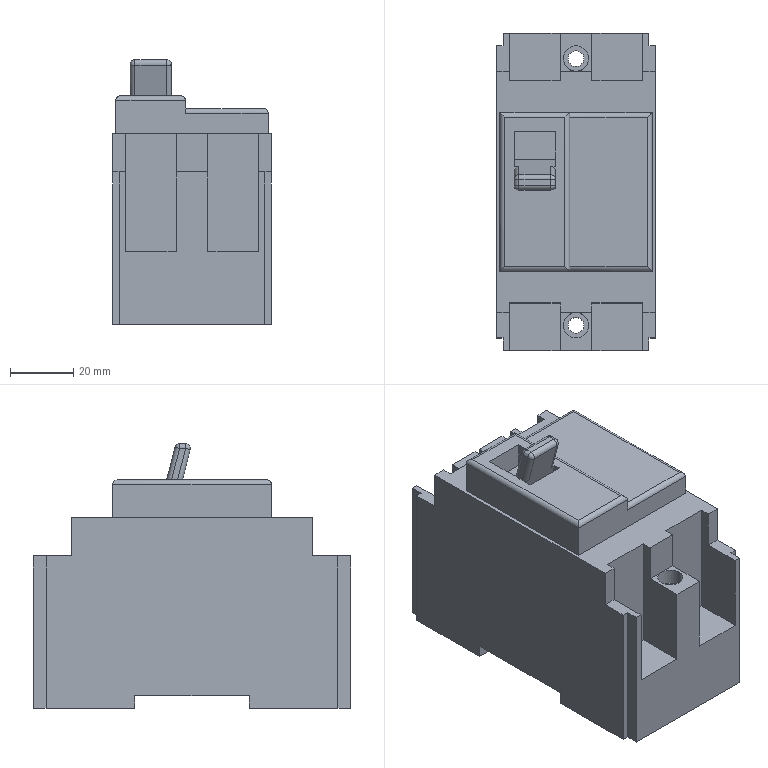Part | SolidWorks | features BaseBody 1 | 1 solid | 95 faces | box 50 x 100 x 83.38 mm | volume 271200 mm3 | plane 68 | cylinder 23 | sphere 4 | commonest cylinder face diameters 3 x15 5 x4 8 x4